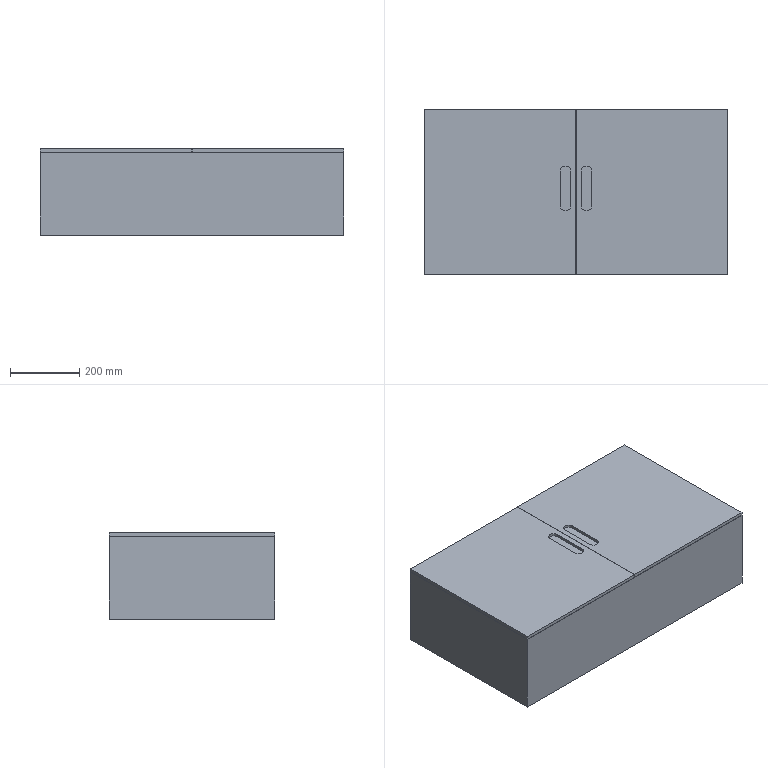Part | STEP file | Electrical control box | 3 solids | 28 faces | box 880 x 480 x 250 mm | volume 105113730 mm3 | plane 24 | cylinder 4 | commonest cylinder face diameters 30 x4